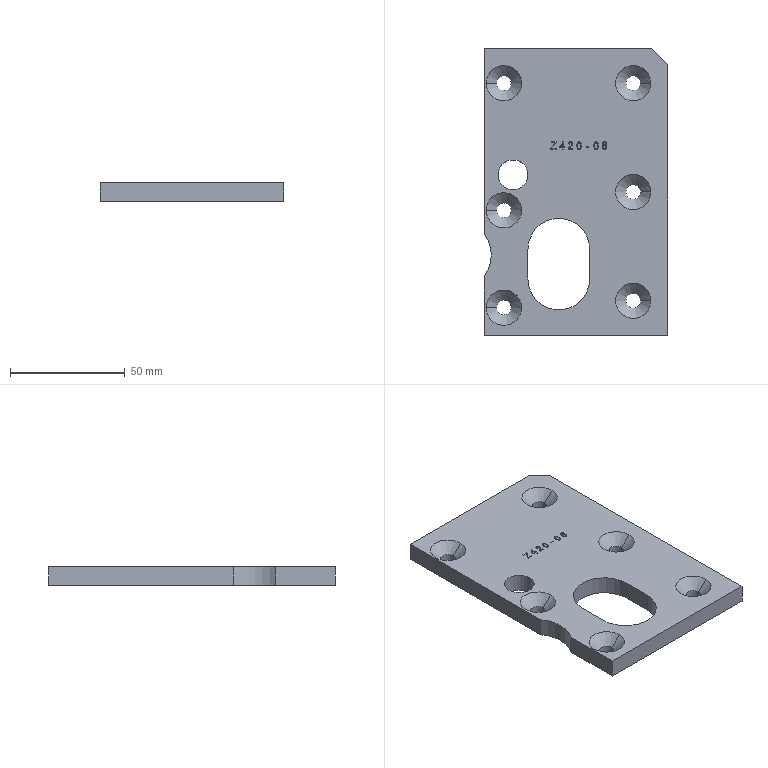Part | Creo | 1 solid | 176 faces | box 80 x 125 x 8 mm | volume 67694 mm3 | other 95 | plane 49 | cylinder 20 | cone 12 | commonest cylinder face diameters 6.4 x12 13 x2 27 x2 1.666 x1 2.89 x1 31 x1